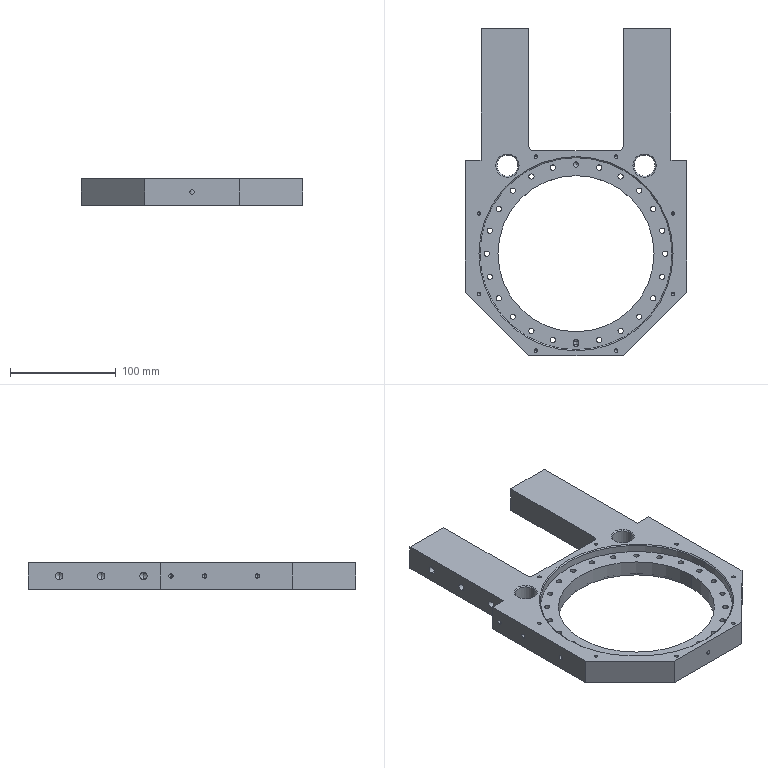Part | SolidWorks | features HoleWzd 11, ICE 7, Chamfer 3, Cut 2, Fillet 2, Extrusion 1 | 1 solid | 193 faces | box 210 x 310 x 25 mm | volume 630464 mm3 | cylinder 111 | cone 58 | plane 24 | commonest cylinder face diameters 5 x48 3.3 x16 4.2 x14 6.8 x12 8.5 x4 20 x4